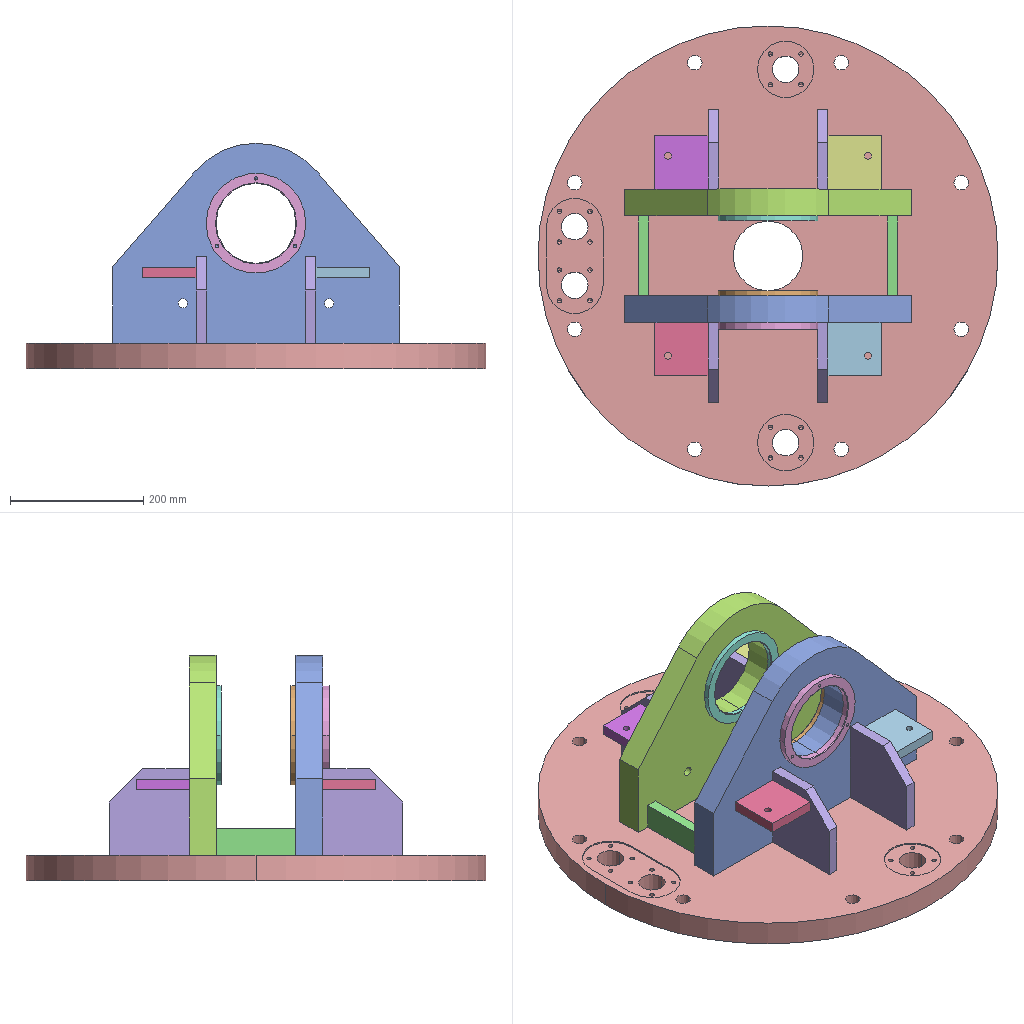Assembly | SolidWorks | 6 different items | 16 placed | box 690 x 690 x 338 mm
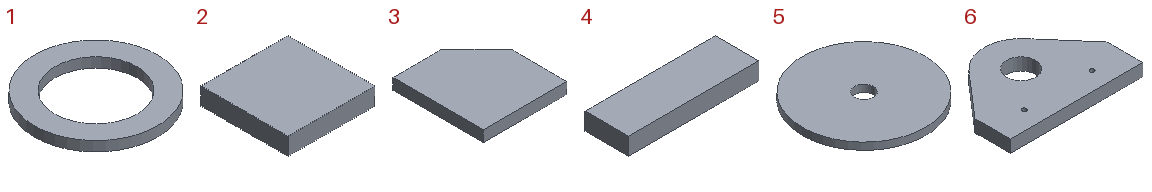Parts list (item | quantity | size | volume | features):
1 | x3 | 150 x 150 x 12 mm | 117810 mm3 | features Extrusion 1
2 | x4 | 80 x 80 x 16 mm | 102400 mm3 | features Chamfer 1, Extrusion 1
3 | x4 | 120 x 130 x 16 mm | 229600 mm3 | features Chamfer 1, Extrusion 1
4 | x2 | 120 x 40 x 16 mm | 76800 mm3 | features Extrusion 1
5 | x1 | 690 x 690 x 40 mm | 14610762 mm3 | features Extrusion 1, ICE 1
6 | x2 | 430 x 300 x 40 mm | 3646282 mm3 | features Extrusion 1, HoleWzd 1, ICE 1
Mates (type | each side: item.copy, entity, surface, feature):
Coincident | 5.1 face plane | 6.1 face plane
Concentric | 6.1 face | 6.2 face
Coincident | 5.1 face plane | 6.2 face plane
DistanceDim | 6.2 face plane | 6.1 face plane
Symmetric | 6.1 face plane | 6.2 face plane | assembly plane
Coincident | 6.1 face plane | 1.1 face plane
Concentric | 6.1 face | 1.1 face
Coincident | 6.1 face plane | 1.2 face plane
Concentric | 6.1 face | 1.2 face
Coincident | 6.2 face plane | 1.3 face plane
Concentric | 6.2 face | 1.3 face
Coincident | 6.2 face plane | 3.1 face plane Boss-Extrude1
Coincident | 5.1 face plane | 3.1 face plane Boss-Extrude1
Coincident | 6.2 face plane | 3.2 face plane Boss-Extrude1
Coincident | 5.1 face plane | 3.2 face plane Boss-Extrude1
DistanceDim | 3.1 face plane Boss-Extrude1 | 3.2 face plane Boss-Extrude1
Width | 3.2 face plane Boss-Extrude1 | 3.1 face plane Boss-Extrude1 | 5.1 face cylinder
Coincident | 5.1 face plane | 4.1 face plane Boss-Extrude1
Coincident | 6.2 face plane | 4.1 face plane Boss-Extrude1
Coincident | 5.1 plane | 6.2 plane
DistanceDim | 4.2 face plane Boss-Extrude1 | 6.2 face plane
DistanceDim | 2.1 face plane | 5.1 face plane
Coincident | 6.2 face plane | 2.2 face plane
Coincident | 2.1 face plane | 2.2 face plane
Coincident | 2.1 face plane | 2.3 face plane
Coincident | 2.4 face plane | 2.2 face plane
Coincident | 3.2 face plane Boss-Extrude1 | 2.2 face plane
Coincident | 2.1 face plane | 3.3 face plane Boss-Extrude1
Coincident | 6.1 face plane | 2.1 face plane
Coincident | 3.4 face plane Boss-Extrude1 | 2.3 face plane
Coincident | 6.1 face plane | 2.3 face plane
Coincident | 2.4 face plane | 3.1 face plane Boss-Extrude1
Coincident | 6.2 face plane | 2.4 face plane